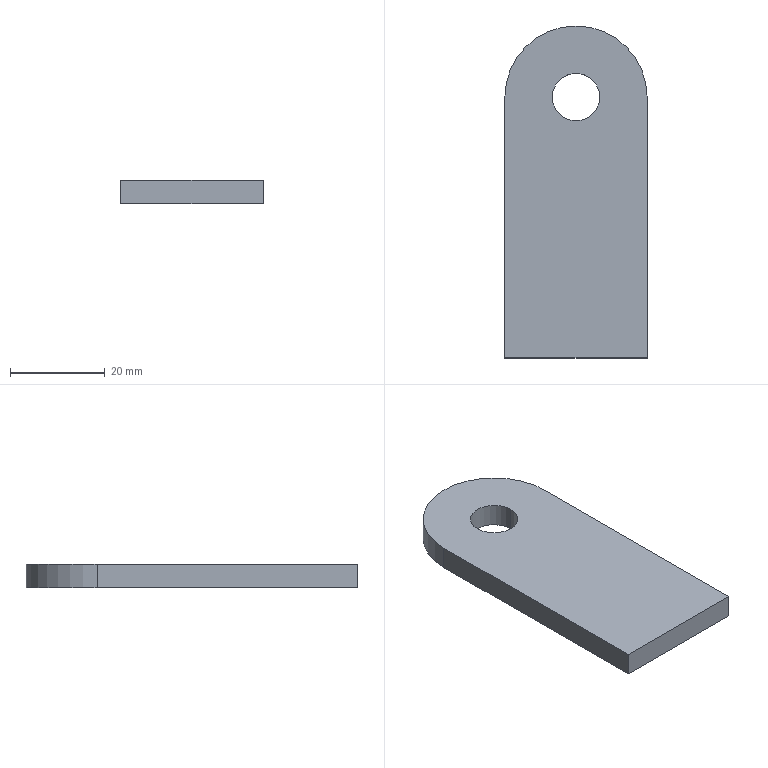Part | SolidWorks | features Extrusion 1 | 1 solid | 8 faces | box 30 x 70 x 5 mm | volume 9624 mm3 | plane 5 | cylinder 3 | commonest cylinder face diameters 10 x2 30 x1
STEP:
#1=CARTESIAN_POINT('',(10.,55.,5.));
#2=VERTEX_POINT('',#1);
#3=CARTESIAN_POINT('',(20.,55.,5.));
#4=VERTEX_POINT('',#3);
#5=CARTESIAN_POINT('',(15.,55.,5.));
#6=DIRECTION('',(0.,0.,1.));
#7=DIRECTION('',(1.,0.,0.));
#8=AXIS2_PLACEMENT_3D('',#5,#6,#7);
#9=CIRCLE('',#8,5.);
#10=EDGE_CURVE('',#2,#4,#9,.T.);
#11=ORIENTED_EDGE('',*,*,#10,.T.);
#12=CARTESIAN_POINT('',(20.,55.,0.));
#13=VERTEX_POINT('',#12);
#14=CARTESIAN_POINT('',(20.,55.,5.));
#15=DIRECTION('',(0.,0.,-1.));
#16=VECTOR('',#15,1000.);
#17=LINE('',#14,#16);
#18=EDGE_CURVE('',#4,#13,#17,.T.);
#19=ORIENTED_EDGE('',*,*,#18,.T.);
#20=CARTESIAN_POINT('',(10.,55.,0.));
#21=VERTEX_POINT('',#20);
#22=CARTESIAN_POINT('',(15.,55.,0.));
#23=DIRECTION('',(0.,0.,1.));
#24=DIRECTION('',(1.,0.,0.));
#25=AXIS2_PLACEMENT_3D('',#22,#23,#24);
#26=CIRCLE('',#25,5.);
#27=EDGE_CURVE('',#21,#13,#26,.T.);
#28=ORIENTED_EDGE('',*,*,#27,.F.);
#29=CARTESIAN_POINT('',(10.,55.,5.));
#30=DIRECTION('',(0.,0.,-1.));
#31=VECTOR('',#30,1000.);
#32=LINE('',#29,#31);
#33=EDGE_CURVE('',#2,#21,#32,.T.);
#34=ORIENTED_EDGE('',*,*,#33,.F.);
#35=EDGE_LOOP('',(#11,#19,#28,#34));
#36=FACE_OUTER_BOUND('',#35,.T.);
#37=CARTESIAN_POINT('',(15.,55.,5.));
#38=DIRECTION('',(0.,0.,-1.));
#39=DIRECTION('',(-1.,0.,0.));
#40=AXIS2_PLACEMENT_3D('',#37,#38,#39);
#41=CYLINDRICAL_SURFACE('',#40,5.);
#42=ADVANCED_FACE('',(#36),#41,.F.);
#43=CARTESIAN_POINT('',(0.,55.,5.));
#44=VERTEX_POINT('',#43);
#45=CARTESIAN_POINT('',(0.,0.,5.));
#46=VERTEX_POINT('',#45);
#47=CARTESIAN_POINT('',(0.,0.,5.));
#48=DIRECTION('',(0.,-1.,0.));
#49=VECTOR('',#48,1000.);
#50=LINE('',#47,#49);
#51=EDGE_CURVE('',#44,#46,#50,.T.);
#52=ORIENTED_EDGE('',*,*,#51,.T.);
#53=CARTESIAN_POINT('',(30.,0.,5.));
#54=VERTEX_POINT('',#53);
#55=CARTESIAN_POINT('',(0.,0.,5.));
#56=DIRECTION('',(1.,0.,0.));
#57=VECTOR('',#56,1000.);
#58=LINE('',#55,#57);
#59=EDGE_CURVE('',#46,#54,#58,.T.);
#60=ORIENTED_EDGE('',*,*,#59,.T.);
#61=CARTESIAN_POINT('',(30.,55.,5.));
#62=VERTEX_POINT('',#61);
#63=CARTESIAN_POINT('',(30.,0.,5.));
#64=DIRECTION('',(0.,1.,0.));
#65=VECTOR('',#64,1000.);
#66=LINE('',#63,#65);
#67=EDGE_CURVE('',#54,#62,#66,.T.);
#68=ORIENTED_EDGE('',*,*,#67,.T.);
#69=CARTESIAN_POINT('',(15.,55.,5.));
#70=DIRECTION('',(0.,0.,1.));
#71=DIRECTION('',(1.,0.,0.));
#72=AXIS2_PLACEMENT_3D('',#69,#70,#71);
#73=CIRCLE('',#72,15.);
#74=EDGE_CURVE('',#62,#44,#73,.T.);
#75=ORIENTED_EDGE('',*,*,#74,.T.);
#76=EDGE_LOOP('',(#52,#60,#68,#75));
#77=FACE_OUTER_BOUND('',#76,.T.);
#78=ORIENTED_EDGE('',*,*,#10,.F.);
#79=CARTESIAN_POINT('',(15.,55.,5.));
#80=DIRECTION('',(0.,0.,1.));
#81=DIRECTION('',(1.,0.,0.));
#82=AXIS2_PLACEMENT_3D('',#79,#80,#81);
#83=CIRCLE('',#82,5.);
#84=EDGE_CURVE('',#4,#2,#83,.T.);
#85=ORIENTED_EDGE('',*,*,#84,.F.);
#86=EDGE_LOOP('',(#78,#85));
#87=FACE_BOUND('',#86,.T.);
#88=CARTESIAN_POINT('',(15.,55.,5.));
#89=DIRECTION('',(0.,0.,1.));
#90=DIRECTION('',(1.,0.,0.));
#91=AXIS2_PLACEMENT_3D('',#88,#89,#90);
#92=PLANE('',#91);
#93=ADVANCED_FACE('',(#77,#87),#92,.T.);
#94=CARTESIAN_POINT('',(0.,55.,0.));
#95=VERTEX_POINT('',#94);
#96=CARTESIAN_POINT('',(0.,0.,0.));
#97=VERTEX_POINT('',#96);
#98=CARTESIAN_POINT('',(0.,0.,0.));
#99=DIRECTION('',(0.,-1.,0.));
#100=VECTOR('',#99,1000.);
#101=LINE('',#98,#100);
#102=EDGE_CURVE('',#95,#97,#101,.T.);
#103=ORIENTED_EDGE('',*,*,#102,.F.);
#104=CARTESIAN_POINT('',(30.,55.,0.));
#105=VERTEX_POINT('',#104);
#106=CARTESIAN_POINT('',(15.,55.,0.));
#107=DIRECTION('',(0.,0.,1.));
#108=DIRECTION('',(1.,0.,0.));
#109=AXIS2_PLACEMENT_3D('',#106,#107,#108);
#110=CIRCLE('',#109,15.);
#111=EDGE_CURVE('',#105,#95,#110,.T.);
#112=ORIENTED_EDGE('',*,*,#111,.F.);
#113=CARTESIAN_POINT('',(30.,0.,0.));
#114=VERTEX_POINT('',#113);
#115=CARTESIAN_POINT('',(30.,0.,0.));
#116=DIRECTION('',(0.,1.,0.));
#117=VECTOR('',#116,1000.);
#118=LINE('',#115,#117);
#119=EDGE_CURVE('',#114,#105,#118,.T.);
#120=ORIENTED_EDGE('',*,*,#119,.F.);
#121=CARTESIAN_POINT('',(0.,0.,0.));
#122=DIRECTION('',(1.,0.,0.));
#123=VECTOR('',#122,1000.);
#124=LINE('',#121,#123);
#125=EDGE_CURVE('',#97,#114,#124,.T.);
#126=ORIENTED_EDGE('',*,*,#125,.F.);
#127=EDGE_LOOP('',(#103,#112,#120,#126));
#128=FACE_OUTER_BOUND('',#127,.T.);
#129=ORIENTED_EDGE('',*,*,#27,.T.);
#130=CARTESIAN_POINT('',(15.,55.,0.));
#131=DIRECTION('',(0.,0.,1.));
#132=DIRECTION('',(1.,0.,0.));
#133=AXIS2_PLACEMENT_3D('',#130,#131,#132);
#134=CIRCLE('',#133,5.);
#135=EDGE_CURVE('',#13,#21,#134,.T.);
#136=ORIENTED_EDGE('',*,*,#135,.T.);
#137=EDGE_LOOP('',(#129,#136));
#138=FACE_BOUND('',#137,.T.);
#139=CARTESIAN_POINT('',(15.,55.,0.));
#140=DIRECTION('',(0.,0.,1.));
#141=DIRECTION('',(1.,0.,0.));
#142=AXIS2_PLACEMENT_3D('',#139,#140,#141);
#143=PLANE('',#142);
#144=ADVANCED_FACE('',(#128,#138),#143,.F.);
#145=ORIENTED_EDGE('',*,*,#102,.T.);
#146=CARTESIAN_POINT('',(0.,0.,5.));
#147=DIRECTION('',(0.,0.,-1.));
#148=VECTOR('',#147,1000.);
#149=LINE('',#146,#148);
#150=EDGE_CURVE('',#46,#97,#149,.T.);
#151=ORIENTED_EDGE('',*,*,#150,.F.);
#152=ORIENTED_EDGE('',*,*,#51,.F.);
#153=CARTESIAN_POINT('',(0.,55.,5.));
#154=DIRECTION('',(0.,0.,-1.));
#155=VECTOR('',#154,1000.);
#156=LINE('',#153,#155);
#157=EDGE_CURVE('',#44,#95,#156,.T.);
#158=ORIENTED_EDGE('',*,*,#157,.T.);
#159=EDGE_LOOP('',(#145,#151,#152,#158));
#160=FACE_OUTER_BOUND('',#159,.T.);
#161=CARTESIAN_POINT('',(0.,0.,5.));
#162=DIRECTION('',(1.,0.,0.));
#163=DIRECTION('',(0.,1.,0.));
#164=AXIS2_PLACEMENT_3D('',#161,#162,#163);
#165=PLANE('',#164);
#166=ADVANCED_FACE('',(#160),#165,.F.);
#167=ORIENTED_EDGE('',*,*,#125,.T.);
#168=CARTESIAN_POINT('',(30.,0.,5.));
#169=DIRECTION('',(0.,0.,-1.));
#170=VECTOR('',#169,1000.);
#171=LINE('',#168,#170);
#172=EDGE_CURVE('',#54,#114,#171,.T.);
#173=ORIENTED_EDGE('',*,*,#172,.F.);
#174=ORIENTED_EDGE('',*,*,#59,.F.);
#175=ORIENTED_EDGE('',*,*,#150,.T.);
#176=EDGE_LOOP('',(#167,#173,#174,#175));
#177=FACE_OUTER_BOUND('',#176,.T.);
#178=CARTESIAN_POINT('',(0.,0.,5.));
#179=DIRECTION('',(0.,1.,0.));
#180=DIRECTION('',(0.,0.,1.));
#181=AXIS2_PLACEMENT_3D('',#178,#179,#180);
#182=PLANE('',#181);
#183=ADVANCED_FACE('',(#177),#182,.F.);
#184=ORIENTED_EDGE('',*,*,#119,.T.);
#185=CARTESIAN_POINT('',(30.,55.,5.));
#186=DIRECTION('',(0.,0.,-1.));
#187=VECTOR('',#186,1000.);
#188=LINE('',#185,#187);
#189=EDGE_CURVE('',#62,#105,#188,.T.);
#190=ORIENTED_EDGE('',*,*,#189,.F.);
#191=ORIENTED_EDGE('',*,*,#67,.F.);
#192=ORIENTED_EDGE('',*,*,#172,.T.);
#193=EDGE_LOOP('',(#184,#190,#191,#192));
#194=FACE_OUTER_BOUND('',#193,.T.);
#195=CARTESIAN_POINT('',(30.,0.,5.));
#196=DIRECTION('',(-1.,0.,0.));
#197=DIRECTION('',(0.,-1.,0.));
#198=AXIS2_PLACEMENT_3D('',#195,#196,#197);
#199=PLANE('',#198);
#200=ADVANCED_FACE('',(#194),#199,.F.);
#201=ORIENTED_EDGE('',*,*,#111,.T.);
#202=ORIENTED_EDGE('',*,*,#157,.F.);
#203=ORIENTED_EDGE('',*,*,#74,.F.);
#204=ORIENTED_EDGE('',*,*,#189,.T.);
#205=EDGE_LOOP('',(#201,#202,#203,#204));
#206=FACE_OUTER_BOUND('',#205,.T.);
#207=CARTESIAN_POINT('',(15.,55.,5.));
#208=DIRECTION('',(0.,0.,-1.));
#209=DIRECTION('',(-1.,0.,0.));
#210=AXIS2_PLACEMENT_3D('',#207,#208,#209);
#211=CYLINDRICAL_SURFACE('',#210,15.);
#212=ADVANCED_FACE('',(#206),#211,.T.);
#213=ORIENTED_EDGE('',*,*,#18,.F.);
#214=ORIENTED_EDGE('',*,*,#84,.T.);
#215=ORIENTED_EDGE('',*,*,#33,.T.);
#216=ORIENTED_EDGE('',*,*,#135,.F.);
#217=EDGE_LOOP('',(#213,#214,#215,#216));
#218=FACE_OUTER_BOUND('',#217,.T.);
#219=CARTESIAN_POINT('',(15.,55.,5.));
#220=DIRECTION('',(0.,0.,-1.));
#221=DIRECTION('',(-1.,0.,0.));
#222=AXIS2_PLACEMENT_3D('',#219,#220,#221);
#223=CYLINDRICAL_SURFACE('',#222,5.);
#224=ADVANCED_FACE('',(#218),#223,.F.);
#225=CLOSED_SHELL('',(#42,#93,#144,#166,#183,#200,#212,#224));
#226=MANIFOLD_SOLID_BREP('',#225);
#227=CARTESIAN_POINT('',(0.,0.,0.));
#228=DIRECTION('',(0.,0.,1.));
#229=DIRECTION('',(1.,0.,0.));
#230=AXIS2_PLACEMENT_3D('',#227,#228,#229);
#231=(LENGTH_UNIT()NAMED_UNIT(*)SI_UNIT(.MILLI.,.METRE.));
#232=UNCERTAINTY_MEASURE_WITH_UNIT(LENGTH_MEASURE(0.00001),#231,'','');
#233=(NAMED_UNIT(*)PLANE_ANGLE_UNIT()SI_UNIT($,.RADIAN.));
#234=(NAMED_UNIT(*)SI_UNIT($,.STERADIAN.)SOLID_ANGLE_UNIT());
#235=(GEOMETRIC_REPRESENTATION_CONTEXT(3)GLOBAL_UNCERTAINTY_ASSIGNED_CONTEXT((#232))GLOBAL_UNIT_ASSIGNED_CONTEXT((#231,#233,#234))REPRESENTATION_CONTEXT('',''));
#236=ADVANCED_BREP_SHAPE_REPRESENTATION('',(#226,#230),#235);